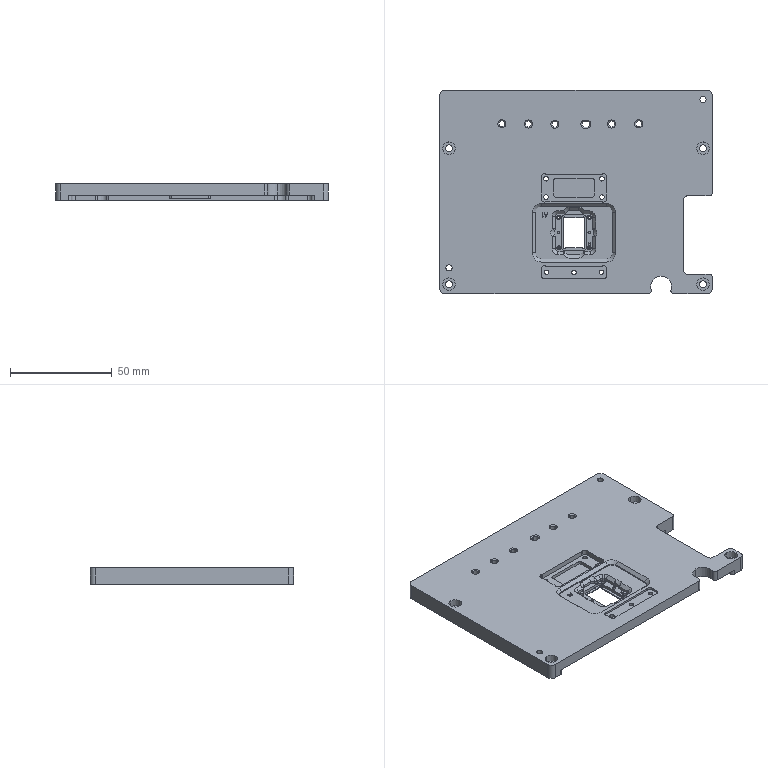NC program | NX | posted with a generic post | part box 134 x 100 x 8 mm
Lines 3064 to 4014 of 16793:
(ZLEVEL_PROFILE_COPY_COPY_COPY_1_COPY_COPY_1_COPY_COPY_COPY_1_COPY_COPY_COPY_1 )
N6066 T17 M6
N6068 G54
N6070 G17 G0 G90 X-14.25 Y-0.808 S9500 M3
N6072 G43 Z30. H17
N6074 Z-0.247
N6076 G94 G1 X-14.85 Y-1.155 F1000.
N6078 G3 X-15.05 Y-1.501 R0.4
N6080 G1 Y-2.49 F1100.
N6082 G2 X-15.074 Y-2.819 R2.3
N6084 X-14.802 Y-2.8 R2.
N6086 G1 X-13.751
N6088 G3 X-13.405 Y-2.6 R0.4
N6090 G1 X-13.058 Y-2.
N6092 G0 X-14.25 Y-0.808 Z-0.436
N6094 G1 X-14.85 Y-1.155 F1000.
N6096 G3 X-15.05 Y-1.501 R0.4
N6098 G1 Y-2.49 F1100.
N6100 G2 X-15.074 Y-2.819 R2.3
N6102 X-14.802 Y-2.8 R2.
N6104 G1 X-13.751
N6106 G3 X-13.405 Y-2.6 R0.4
N6108 G1 X-13.058 Y-2.
N6110 G0 X-14.25 Y-0.808 Z-0.624
N6112 G1 X-14.85 Y-1.155 F1000.
N6114 G3 X-15.05 Y-1.501 R0.4
N6116 G1 Y-2.49 F1100.
N6118 G2 X-15.074 Y-2.819 R2.3
N6120 X-14.802 Y-2.8 R2.
N6122 G1 X-13.751
N6124 G3 X-13.405 Y-2.6 R0.4
N6126 G1 X-13.058 Y-2.
N6128 G0 X-14.25 Y-0.808 Z-0.812
N6130 G1 X-14.85 Y-1.155 F1000.
N6132 G3 X-15.05 Y-1.501 R0.4
N6134 G1 Y-2.49 F1100.
N6136 G2 X-15.074 Y-2.819 R2.3
N6138 X-14.802 Y-2.8 R2.
N6140 G1 X-13.751
N6142 G3 X-13.405 Y-2.6 R0.4
N6144 G1 X-13.058 Y-2.
N6146 G0 X-14.25 Y-0.808 Z-1.
N6148 G1 X-14.85 Y-1.155 F1000.
N6150 G3 X-15.05 Y-1.501 R0.4
N6152 G1 Y-2.49 F1100.
N6154 G2 X-15.074 Y-2.819 R2.3
N6156 X-14.802 Y-2.8 R2.
N6158 G1 X-13.751
N6160 G3 X-13.405 Y-2.6 R0.4
N6162 G1 X-13.058 Y-2.
N6164 G0 X-14.25 Y-0.808 Z-1.247
N6166 G1 X-14.85 Y-1.155 F1000.
N6168 G3 X-15.05 Y-1.501 R0.4
N6170 G1 Y-2.49 F1100.
N6172 G2 X-15.074 Y-2.819 R2.3
N6174 X-14.802 Y-2.8 R2.
N6176 G1 X-13.751
N6178 G3 X-13.405 Y-2.6 R0.4
N6180 G1 X-13.058 Y-2.
N6182 G0 X-14.25 Y-0.808 Z-1.436
N6184 G1 X-14.85 Y-1.155 F1000.
N6186 G3 X-15.05 Y-1.501 R0.4
N6188 G1 Y-2.49 F1100.
N6190 G2 X-15.074 Y-2.819 R2.3
N6192 X-14.802 Y-2.8 R2.
N6194 G1 X-13.751
N6196 G3 X-13.405 Y-2.6 R0.4
N6198 G1 X-13.058 Y-2.
N6200 G0 X-14.25 Y-0.808 Z-1.76
N6202 G1 X-14.85 Y-1.155 F1000.
N6204 G3 X-15.05 Y-1.501 R0.4
N6206 G1 Y-2.49 F1100.
N6208 G2 X-15.074 Y-2.819 R2.3
N6210 X-14.802 Y-2.8 R2.
N6212 G1 X-13.751
N6214 G3 X-13.405 Y-2.6 R0.4
N6216 G1 X-13.058 Y-2.
N6218 G0 X-14.25 Y-0.808 Z-2.
N6220 G1 X-14.85 Y-1.155 F1000.
N6222 G3 X-15.05 Y-1.501 R0.4
N6224 G1 Y-2.49 F1100.
N6226 G2 X-15.074 Y-2.819 R2.3
N6228 X-14.802 Y-2.8 R2.
N6230 G1 X-13.751
N6232 G3 X-13.405 Y-2.6 R0.4
N6234 G1 X-13.058 Y-2.
N6236 G0 X-14.25 Y-0.808 Z-2.1
N6238 G1 X-14.85 Y-1.155 F1000.
N6240 G3 X-15.05 Y-1.501 R0.4
N6242 G1 Y-2.49 F1100.
N6244 G2 X-15.074 Y-2.819 R2.3
N6246 X-14.802 Y-2.8 R2.
N6248 G1 X-13.751
N6250 G3 X-13.405 Y-2.6 R0.4
N6252 G1 X-13.058 Y-2.
N6254 G0 X-14.25 Y-0.808 Z-2.267
N6256 G1 X-14.85 Y-1.155 F1000.
N6258 G3 X-15.05 Y-1.501 R0.4
N6260 G1 Y-2.49 F1100.
N6262 G2 X-15.074 Y-2.819 R2.3
N6264 X-14.802 Y-2.8 R2.
N6266 G1 X-13.751
N6268 G3 X-13.405 Y-2.6 R0.4
N6270 G1 X-13.058 Y-2.
N6272 G0 X-14.25 Y-0.808 Z-2.433
N6274 G1 X-14.85 Y-1.155 F1000.
N6276 G3 X-15.05 Y-1.501 R0.4
N6278 G1 Y-2.49 F1100.
N6280 G2 X-15.074 Y-2.819 R2.3
N6282 X-14.802 Y-2.8 R2.
N6284 G1 X-13.751
N6286 G3 X-13.405 Y-2.6 R0.4
N6288 G1 X-13.058 Y-2.
N6290 G0 X-14.25 Y-0.808 Z-2.6
N6292 G1 X-14.85 Y-1.155 F1000.
N6294 G3 X-15.05 Y-1.501 R0.4
N6296 G1 Y-2.49 F1100.
N6298 G2 X-15.074 Y-2.819 R2.3
N6300 X-14.802 Y-2.8 R2.
N6302 G1 X-13.751
N6304 G3 X-13.405 Y-2.6 R0.4
N6306 G1 X-13.058 Y-2.
N6308 G0 Z30.
N6310 X-8.2 Y1.492
N6312 Z-2.825
N6314 G1 X-8.8 Y1.145 F1000.
N6316 G3 X-9. Y0.799 R0.4
N6318 G1 Y-0.5 F1100.
N6320 X-7.701
N6322 G3 X-7.355 Y-0.3 R0.4
N6324 G1 X-7.008 Y0.3
N6326 G0 X-8.2 Y1.492 Z-3.05
N6328 G1 X-8.8 Y1.145 F1000.
N6330 G3 X-9. Y0.799 R0.4
N6332 G1 Y-0.5 F1100.
N6334 X-7.701
N6336 G3 X-7.355 Y-0.3 R0.4
N6338 G1 X-7.008 Y0.3
N6340 G0 X-8.2 Y1.492 Z-3.275
N6342 G1 X-8.8 Y1.145 F1000.
N6344 G3 X-9. Y0.799 R0.4
N6346 G1 Y-0.5 F1100.
N6348 X-7.701
N6350 G3 X-7.355 Y-0.3 R0.4
N6352 G1 X-7.008 Y0.3
N6354 G0 X-8.2 Y1.492 Z-3.5
N6356 G1 X-8.8 Y1.145 F1000.
N6358 G3 X-9. Y0.799 R0.4
N6360 G1 Y-0.5 F1100.
N6362 X-7.701
N6364 G3 X-7.355 Y-0.3 R0.4
N6366 G1 X-7.008 Y0.3
N6368 G0 X-8.2 Y1.492 Z-3.85
N6370 G1 X-8.8 Y1.145 F1000.
N6372 G3 X-9. Y0.799 R0.4
N6374 G1 Y-0.5 F1100.
N6376 X-7.701
N6378 G3 X-7.355 Y-0.3 R0.4
N6380 G1 X-7.008 Y0.3
N6382 G0 X-8.2 Y1.492 Z-4.05
N6384 G1 X-8.8 Y1.145 F1000.
N6386 G3 X-9. Y0.799 R0.4
N6388 G1 Y-0.5 F1100.
N6390 X-7.701
N6392 G3 X-7.355 Y-0.3 R0.4
N6394 G1 X-7.008 Y0.3
N6396 G0 X-8.2 Y1.492 Z-4.2
N6398 G1 X-8.8 Y1.145 F1000.
N6400 G3 X-9. Y0.799 R0.4
N6402 G1 Y-0.5 F1100.
N6404 X-7.701
N6406 G3 X-7.355 Y-0.3 R0.4
N6408 G1 X-7.008 Y0.3
N6410 G0 Z30.
N6412 X11.058 Y-2.
N6414 Z-0.247
N6416 G1 X11.404 Y-2.6 F1000.
N6418 G3 X11.751 Y-2.8 R0.4
N6420 G1 X12.74 F1100.
N6422 G2 X13.074 Y-2.824 R2.3
N6424 X13.05 Y-2.49 R2.3
N6426 G1 Y-1.501
N6428 G3 X12.85 Y-1.154 R0.4
N6430 G1 X12.25 Y-0.808
N6432 G0 X11.058 Y-2. Z-0.436
N6434 G1 X11.404 Y-2.6 F1000.
N6436 G3 X11.751 Y-2.8 R0.4
N6438 G1 X12.74 F1100.
N6440 G2 X13.074 Y-2.824 R2.3
N6442 X13.05 Y-2.49 R2.3
N6444 G1 Y-1.501
N6446 G3 X12.85 Y-1.154 R0.4
N6448 G1 X12.25 Y-0.808
N6450 G0 X11.057 Y-2. Z-0.624
N6452 G1 X11.404 Y-2.6 F1000.
N6454 G3 X11.75 Y-2.8 R0.4
N6456 G1 X12.74 F1100.
N6458 G2 X13.074 Y-2.824 R2.3
N6460 X13.05 Y-2.49 R2.3
N6462 G1 Y-1.5
N6464 G3 X12.85 Y-1.154 R0.4
N6466 G1 X12.25 Y-0.807
N6468 G0 X11.057 Y-2. Z-0.812
N6470 G1 X11.404 Y-2.6 F1000.
N6472 G3 X11.75 Y-2.8 R0.4
N6474 G1 X12.74 F1100.
N6476 G2 X13.074 Y-2.824 R2.3
N6478 X13.05 Y-2.49 R2.3
N6480 G1 Y-1.5
N6482 G3 X12.85 Y-1.154 R0.4
N6484 G1 X12.25 Y-0.807
N6486 G0 X11.057 Y-2. Z-1.
N6488 G1 X11.404 Y-2.6 F1000.
N6490 G3 X11.75 Y-2.8 R0.4
N6492 G1 X12.74 F1100.
N6494 G2 X13.074 Y-2.824 R2.3
N6496 X13.05 Y-2.49 R2.3
N6498 G1 Y-1.5
N6500 G3 X12.85 Y-1.154 R0.4
N6502 G1 X12.25 Y-0.807
N6504 G0 X11.057 Y-2. Z-1.247
N6506 G1 X11.403 Y-2.6 F1000.
N6508 G3 X11.75 Y-2.8 R0.4
N6510 G1 X12.74 F1100.
N6512 G2 X13.074 Y-2.824 R2.3
N6514 X13.05 Y-2.49 R2.3
N6516 G1 Y-1.5
N6518 G3 X12.85 Y-1.153 R0.4
N6520 G1 X12.25 Y-0.807
N6522 G0 X11.057 Y-2. Z-1.436
N6524 G1 X11.403 Y-2.6 F1000.
N6526 G3 X11.749 Y-2.8 R0.4
N6528 G1 X12.74 F1100.
N6530 G2 X13.074 Y-2.824 R2.3
N6532 X13.05 Y-2.49 R2.3
N6534 G1 Y-1.499
N6536 G3 X12.85 Y-1.153 R0.4
N6538 G1 X12.25 Y-0.807
N6540 G0 X11.056 Y-2. Z-1.76
N6542 G1 X11.403 Y-2.6 F1000.
N6544 G3 X11.749 Y-2.8 R0.4
N6546 G1 X12.74 F1100.
N6548 G2 X13.074 Y-2.824 R2.3
N6550 X13.05 Y-2.49 R2.3
N6552 G1 Y-1.499
N6554 G3 X12.85 Y-1.153 R0.4
N6556 G1 X12.25 Y-0.806
N6558 G0 X11.056 Y-2. Z-2.
N6560 G1 X11.402 Y-2.6 F1000.
N6562 G3 X11.749 Y-2.8 R0.4
N6564 G1 X12.74 F1100.
N6566 G2 X13.074 Y-2.824 R2.3
N6568 X13.05 Y-2.49 R2.3
N6570 G1 Y-1.499
N6572 G3 X12.85 Y-1.152 R0.4
N6574 G1 X12.25 Y-0.806
N6576 G0 X11.056 Y-2. Z-2.1
N6578 G1 X11.402 Y-2.6 F1000.
N6580 G3 X11.749 Y-2.8 R0.4
N6582 G1 X12.74 F1100.
N6584 G2 X13.074 Y-2.824 R2.3
N6586 X13.05 Y-2.49 R2.3
N6588 G1 Y-1.499
N6590 G3 X12.85 Y-1.152 R0.4
N6592 G1 X12.25 Y-0.806
N6594 G0 X11.056 Y-2. Z-2.267
N6596 G1 X11.402 Y-2.6 F1000.
N6598 G3 X11.749 Y-2.8 R0.4
N6600 G1 X12.74 F1100.
N6602 G2 X13.074 Y-2.824 R2.3
N6604 X13.05 Y-2.49 R2.3
N6606 G1 Y-1.499
N6608 G3 X12.85 Y-1.152 R0.4
N6610 G1 X12.25 Y-0.806
N6612 G0 X11.056 Y-2. Z-2.433
N6614 G1 X11.402 Y-2.6 F1000.
N6616 G3 X11.748 Y-2.8 R0.4
N6618 G1 X12.74 F1100.
N6620 G2 X13.074 Y-2.824 R2.3
N6622 X13.05 Y-2.49 R2.3
N6624 G1 Y-1.498
N6626 G3 X12.85 Y-1.152 R0.4
N6628 G1 X12.25 Y-0.806
N6630 G0 X11.055 Y-2. Z-2.6
N6632 G1 X11.402 Y-2.6 F1000.
N6634 G3 X11.748 Y-2.8 R0.4
N6636 G1 X12.74 F1100.
N6638 G2 X13.074 Y-2.824 R2.3
N6640 X13.05 Y-2.49 R2.3
N6642 G1 Y-1.498
N6644 G3 X12.85 Y-1.152 R0.4
N6646 G1 X12.25 Y-0.805
N6648 G0 Z30.
N6650 X5.008 Y0.3
N6652 Z-2.825
N6654 G1 X5.355 Y-0.3 F1000.
N6656 G3 X5.701 Y-0.5 R0.4
N6658 G1 X7. F1100.
N6660 Y0.799
N6662 G3 X6.8 Y1.145 R0.4
N6664 G1 X6.2 Y1.492
N6666 G0 X5.008 Y0.3 Z-3.05
N6668 G1 X5.355 Y-0.3 F1000.
N6670 G3 X5.701 Y-0.5 R0.4
N6672 G1 X7. F1100.
N6674 Y0.799
N6676 G3 X6.8 Y1.145 R0.4
N6678 G1 X6.2 Y1.492
N6680 G0 X5.008 Y0.3 Z-3.275
N6682 G1 X5.355 Y-0.3 F1000.
N6684 G3 X5.701 Y-0.5 R0.4
N6686 G1 X7. F1100.
N6688 Y0.799
N6690 G3 X6.8 Y1.145 R0.4
N6692 G1 X6.2 Y1.492
N6694 G0 X5.008 Y0.3 Z-3.5
N6696 G1 X5.355 Y-0.3 F1000.
N6698 G3 X5.701 Y-0.5 R0.4
N6700 G1 X7. F1100.
N6702 Y0.799
N6704 G3 X6.8 Y1.145 R0.4
N6706 G1 X6.2 Y1.492
N6708 G0 X5.008 Y0.3 Z-3.85
N6710 G1 X5.355 Y-0.3 F1000.
N6712 G3 X5.701 Y-0.5 R0.4
N6714 G1 X7. F1100.
N6716 Y0.799
N6718 G3 X6.8 Y1.145 R0.4
N6720 G1 X6.2 Y1.492
N6722 G0 X5.008 Y0.3 Z-4.05
N6724 G1 X5.355 Y-0.3 F1000.
N6726 G3 X5.701 Y-0.5 R0.4
N6728 G1 X7. F1100.
N6730 Y0.799
N6732 G3 X6.8 Y1.145 R0.4
N6734 G1 X6.2 Y1.492
N6736 G0 X5.008 Y0.3 Z-4.2
N6738 G1 X5.355 Y-0.3 F1000.
N6740 G3 X5.701 Y-0.5 R0.4
N6742 G1 X7. F1100.
N6744 Y0.799
N6746 G3 X6.8 Y1.145 R0.4
N6748 G1 X6.2 Y1.492
N6750 G0 Z30.
N6752 X12.25 Y4.808
N6754 Z-0.247
N6756 G1 X12.85 Y5.155 F1000.
N6758 G3 X13.05 Y5.501 R0.4
N6760 G1 Y6.49 F1100.
N6762 G2 X13.074 Y6.824 R2.3
N6764 X12.74 Y6.8 R2.3
N6766 G1 X11.751
N6768 G3 X11.405 Y6.6 R0.4
N6770 G1 X11.058 Y6.
N6772 G0 X12.25 Y4.808 Z-0.436
N6774 G1 X12.85 Y5.155 F1000.
N6776 G3 X13.05 Y5.501 R0.4
N6778 G1 Y6.49 F1100.
N6780 G2 X13.074 Y6.824 R2.3
N6782 X12.74 Y6.8 R2.3
N6784 G1 X11.751
N6786 G3 X11.405 Y6.6 R0.4
N6788 G1 X11.058 Y6.
N6790 G0 X12.25 Y4.808 Z-0.624
N6792 G1 X12.85 Y5.155 F1000.
N6794 G3 X13.05 Y5.501 R0.4
N6796 G1 Y6.49 F1100.
N6798 G2 X13.074 Y6.824 R2.3
N6800 X12.74 Y6.8 R2.3
N6802 G1 X11.751
N6804 G3 X11.405 Y6.6 R0.4
N6806 G1 X11.058 Y6.
N6808 G0 X12.25 Y4.808 Z-0.812
N6810 G1 X12.85 Y5.155 F1000.
N6812 G3 X13.05 Y5.501 R0.4
N6814 G1 Y6.49 F1100.
N6816 G2 X13.074 Y6.824 R2.3
N6818 X12.74 Y6.8 R2.3
N6820 G1 X11.751
N6822 G3 X11.405 Y6.6 R0.4
N6824 G1 X11.058 Y6.
N6826 G0 X12.25 Y4.808 Z-1.
N6828 G1 X12.85 Y5.155 F1000.
N6830 G3 X13.05 Y5.501 R0.4
N6832 G1 Y6.49 F1100.
N6834 G2 X13.074 Y6.824 R2.3
N6836 X12.74 Y6.8 R2.3
N6838 G1 X11.751
N6840 G3 X11.405 Y6.6 R0.4
N6842 G1 X11.058 Y6.
N6844 G0 X12.25 Y4.808 Z-1.247
N6846 G1 X12.85 Y5.155 F1000.
N6848 G3 X13.05 Y5.501 R0.4
N6850 G1 Y6.49 F1100.
N6852 G2 X13.074 Y6.824 R2.3
N6854 X12.74 Y6.8 R2.3
N6856 G1 X11.751
N6858 G3 X11.405 Y6.6 R0.4
N6860 G1 X11.058 Y6.
N6862 G0 X12.25 Y4.808 Z-1.436
N6864 G1 X12.85 Y5.155 F1000.
N6866 G3 X13.05 Y5.501 R0.4
N6868 G1 Y6.49 F1100.
N6870 G2 X13.074 Y6.824 R2.3
N6872 X12.74 Y6.8 R2.3
N6874 G1 X11.751
N6876 G3 X11.405 Y6.6 R0.4
N6878 G1 X11.058 Y6.
N6880 G0 X12.25 Y4.808 Z-1.76
N6882 G1 X12.85 Y5.155 F1000.
N6884 G3 X13.05 Y5.501 R0.4
N6886 G1 Y6.49 F1100.
N6888 G2 X13.074 Y6.824 R2.3
N6890 X12.74 Y6.8 R2.3
N6892 G1 X11.751
N6894 G3 X11.405 Y6.6 R0.4
N6896 G1 X11.058 Y6.
N6898 G0 X12.25 Y4.808 Z-2.
N6900 G1 X12.85 Y5.155 F1000.
N6902 G3 X13.05 Y5.501 R0.4
N6904 G1 Y6.49 F1100.
N6906 G2 X13.074 Y6.824 R2.3
N6908 X12.74 Y6.8 R2.3
N6910 G1 X11.751
N6912 G3 X11.405 Y6.6 R0.4
N6914 G1 X11.058 Y6.
N6916 G0 X12.25 Y4.808 Z-2.1
N6918 G1 X12.85 Y5.155 F1000.
N6920 G3 X13.05 Y5.501 R0.4
N6922 G1 Y6.49 F1100.
N6924 G2 X13.074 Y6.824 R2.3
N6926 X12.74 Y6.8 R2.3
N6928 G1 X11.751
N6930 G3 X11.405 Y6.6 R0.4
N6932 G1 X11.058 Y6.
N6934 G0 X12.25 Y4.808 Z-2.267
N6936 G1 X12.85 Y5.155 F1000.
N6938 G3 X13.05 Y5.501 R0.4
N6940 G1 Y6.49 F1100.
N6942 G2 X13.074 Y6.824 R2.3
N6944 X12.74 Y6.8 R2.3
N6946 G1 X11.751
N6948 G3 X11.405 Y6.6 R0.4
N6950 G1 X11.058 Y6.
N6952 G0 X12.25 Y4.808 Z-2.433
N6954 G1 X12.85 Y5.155 F1000.
N6956 G3 X13.05 Y5.501 R0.4
N6958 G1 Y6.49 F1100.
N6960 G2 X13.074 Y6.824 R2.3
N6962 X12.74 Y6.8 R2.3
N6964 G1 X11.751
N6966 G3 X11.405 Y6.6 R0.4
N6968 G1 X11.058 Y6.
N6970 G0 X12.25 Y4.808 Z-2.6
N6972 G1 X12.85 Y5.155 F1000.
N6974 G3 X13.05 Y5.501 R0.4
N6976 G1 Y6.49 F1100.
N6978 G2 X13.074 Y6.824 R2.3
N6980 X12.74 Y6.8 R2.3
N6982 G1 X11.751
N6984 G3 X11.405 Y6.6 R0.4
N6986 G1 X11.058 Y6.
N6988 G0 Z30.
N6990 X6.2 Y2.508
N6992 Z-2.825
N6994 G1 X6.8 Y2.855 F1000.
N6996 G3 X7. Y3.201 R0.4
N6998 G1 Y4.5 F1100.
N7000 X5.701
N7002 G3 X5.355 Y4.3 R0.4
N7004 G1 X5.008 Y3.7
N7006 G0 X6.2 Y2.508 Z-3.05
N7008 G1 X6.8 Y2.855 F1000.
N7010 G3 X7. Y3.201 R0.4
N7012 G1 Y4.5 F1100.
N7014 X5.701
N7016 G3 X5.355 Y4.3 R0.4
N7018 G1 X5.008 Y3.7
N7020 G0 X6.2 Y2.508 Z-3.275
N7022 G1 X6.8 Y2.855 F1000.
N7024 G3 X7. Y3.201 R0.4
N7026 G1 Y4.5 F1100.
N7028 X5.701
N7030 G3 X5.355 Y4.3 R0.4
N7032 G1 X5.008 Y3.7
N7034 G0 X6.2 Y2.508 Z-3.5
N7036 G1 X6.8 Y2.855 F1000.
N7038 G3 X7. Y3.201 R0.4
N7040 G1 Y4.5 F1100.
N7042 X5.701
N7044 G3 X5.355 Y4.3 R0.4
N7046 G1 X5.008 Y3.7
N7048 G0 X6.2 Y2.508 Z-3.85
N7050 G1 X6.8 Y2.855 F1000.
N7052 G3 X7. Y3.201 R0.4
N7054 G1 Y4.5 F1100.
N7056 X5.701
N7058 G3 X5.355 Y4.3 R0.4
N7060 G1 X5.008 Y3.7
N7062 G0 X6.2 Y2.508 Z-4.05
N7064 G1 X6.8 Y2.855 F1000.
N7066 G3 X7. Y3.201 R0.4
N7068 G1 Y4.5 F1100.
N7070 X5.701
N7072 G3 X5.355 Y4.3 R0.4
N7074 G1 X5.008 Y3.7
N7076 G0 X6.2 Y2.508 Z-4.2
N7078 G1 X6.8 Y2.855 F1000.
N7080 G3 X7. Y3.201 R0.4
N7082 G1 Y4.5 F1100.
N7084 X5.701
N7086 G3 X5.355 Y4.3 R0.4
N7088 G1 X5.008 Y3.7
N7090 G0 Z30.
N7092 X-13.058 Y6.
N7094 Z-0.247
N7096 G1 X-13.405 Y6.6 F1000.
N7098 G3 X-13.751 Y6.8 R0.4
N7100 G1 X-14.74 F1100.
N7102 G2 X-15.074 Y6.824 R2.3
N7104 X-15.05 Y6.49 R2.3
N7106 G1 Y5.501
N7108 G3 X-14.85 Y5.155 R0.4
N7110 G1 X-14.25 Y4.808
N7112 G0 X-13.058 Y6. Z-0.436
N7114 G1 X-13.405 Y6.6 F1000.
N7116 G3 X-13.751 Y6.8 R0.4
N7118 G1 X-14.74 F1100.
N7120 G2 X-15.074 Y6.824 R2.3
N7122 X-15.05 Y6.49 R2.3
N7124 G1 Y5.501
N7126 G3 X-14.85 Y5.155 R0.4
N7128 G1 X-14.25 Y4.808
N7130 G0 X-13.058 Y6. Z-0.624
N7132 G1 X-13.405 Y6.6 F1000.
N7134 G3 X-13.751 Y6.8 R0.4
N7136 G1 X-14.74 F1100.
N7138 G2 X-15.074 Y6.824 R2.3
N7140 X-15.05 Y6.49 R2.3
N7142 G1 Y5.501
N7144 G3 X-14.85 Y5.155 R0.4
N7146 G1 X-14.25 Y4.808
N7148 G0 X-13.058 Y6. Z-0.812
N7150 G1 X-13.405 Y6.6 F1000.
N7152 G3 X-13.751 Y6.8 R0.4
N7154 G1 X-14.74 F1100.
N7156 G2 X-15.074 Y6.824 R2.3
N7158 X-15.05 Y6.49 R2.3
N7160 G1 Y5.501
N7162 G3 X-14.85 Y5.155 R0.4
N7164 G1 X-14.25 Y4.808
N7166 G0 X-13.058 Y6. Z-1.
N7168 G1 X-13.405 Y6.6 F1000.
N7170 G3 X-13.751 Y6.8 R0.4
N7172 G1 X-14.74 F1100.
N7174 G2 X-15.074 Y6.824 R2.3
N7176 X-15.05 Y6.49 R2.3
N7178 G1 Y5.501
N7180 G3 X-14.85 Y5.155 R0.4
N7182 G1 X-14.25 Y4.808
N7184 G0 X-13.058 Y6. Z-1.247
N7186 G1 X-13.405 Y6.6 F1000.
N7188 G3 X-13.751 Y6.8 R0.4
N7190 G1 X-14.74 F1100.
N7192 G2 X-15.074 Y6.824 R2.3
N7194 X-15.05 Y6.49 R2.3
N7196 G1 Y5.501
N7198 G3 X-14.85 Y5.155 R0.4
N7200 G1 X-14.25 Y4.808
N7202 G0 X-13.058 Y6. Z-1.436
N7204 G1 X-13.405 Y6.6 F1000.
N7206 G3 X-13.751 Y6.8 R0.4
N7208 G1 X-14.74 F1100.
N7210 G2 X-15.074 Y6.824 R2.3
N7212 X-15.05 Y6.49 R2.3
N7214 G1 Y5.501
N7216 G3 X-14.85 Y5.155 R0.4
N7218 G1 X-14.25 Y4.808
N7220 G0 X-13.058 Y6. Z-1.76
N7222 G1 X-13.405 Y6.6 F1000.
N7224 G3 X-13.751 Y6.8 R0.4
N7226 G1 X-14.74 F1100.
N7228 G2 X-15.074 Y6.824 R2.3
N7230 X-15.05 Y6.49 R2.3
N7232 G1 Y5.501
N7234 G3 X-14.85 Y5.155 R0.4
N7236 G1 X-14.25 Y4.808
N7238 G0 X-13.058 Y6. Z-2.
N7240 G1 X-13.405 Y6.6 F1000.
N7242 G3 X-13.751 Y6.8 R0.4
N7244 G1 X-14.74 F1100.
N7246 G2 X-15.074 Y6.824 R2.3
N7248 X-15.05 Y6.49 R2.3
N7250 G1 Y5.501
N7252 G3 X-14.85 Y5.155 R0.4
N7254 G1 X-14.25 Y4.808
N7256 G0 X-13.058 Y6. Z-2.1
N7258 G1 X-13.405 Y6.6 F1000.
N7260 G3 X-13.751 Y6.8 R0.4
N7262 G1 X-14.74 F1100.
N7264 G2 X-15.074 Y6.824 R2.3
N7266 X-15.05 Y6.49 R2.3
N7268 G1 Y5.501
N7270 G3 X-14.85 Y5.155 R0.4
N7272 G1 X-14.25 Y4.808
N7274 G0 X-13.058 Y6. Z-2.267
N7276 G1 X-13.405 Y6.6 F1000.
N7278 G3 X-13.751 Y6.8 R0.4
N7280 G1 X-14.74 F1100.
N7282 G2 X-15.074 Y6.824 R2.3
N7284 X-15.05 Y6.49 R2.3
N7286 G1 Y5.501
N7288 G3 X-14.85 Y5.155 R0.4
N7290 G1 X-14.25 Y4.808
N7292 G0 X-13.058 Y6. Z-2.433
N7294 G1 X-13.405 Y6.6 F1000.
N7296 G3 X-13.751 Y6.8 R0.4
N7298 G1 X-14.74 F1100.
N7300 G2 X-15.074 Y6.824 R2.3
N7302 X-15.05 Y6.49 R2.3
N7304 G1 Y5.501
N7306 G3 X-14.85 Y5.155 R0.4
N7308 G1 X-14.25 Y4.808
N7310 G0 X-13.058 Y6. Z-2.6
N7312 G1 X-13.405 Y6.6 F1000.
N7314 G3 X-13.751 Y6.8 R0.4
N7316 G1 X-14.74 F1100.
N7318 G2 X-15.074 Y6.824 R2.3
N7320 X-15.05 Y6.49 R2.3
N7322 G1 Y5.501
N7324 G3 X-14.85 Y5.155 R0.4
N7326 G1 X-14.25 Y4.808
N7328 G0 Z30.
N7330 X-7.008 Y3.7
N7332 Z-2.825
N7334 G1 X-7.355 Y4.3 F1000.
N7336 G3 X-7.701 Y4.5 R0.4
N7338 G1 X-9. F1100.
N7340 Y3.201
N7342 G3 X-8.8 Y2.855 R0.4
N7344 G1 X-8.2 Y2.508
N7346 G0 X-7.008 Y3.7 Z-3.05
N7348 G1 X-7.355 Y4.3 F1000.
N7350 G3 X-7.701 Y4.5 R0.4
N7352 G1 X-9. F1100.
N7354 Y3.201
N7356 G3 X-8.8 Y2.855 R0.4
N7358 G1 X-8.2 Y2.508
N7360 G0 X-7.008 Y3.7 Z-3.275
N7362 G1 X-7.355 Y4.3 F1000.
N7364 G3 X-7.701 Y4.5 R0.4
N7366 G1 X-9. F1100.
N7368 Y3.201
N7370 G3 X-8.8 Y2.855 R0.4
N7372 G1 X-8.2 Y2.508
N7374 G0 X-7.008 Y3.7 Z-3.5
N7376 G1 X-7.355 Y4.3 F1000.
N7378 G3 X-7.701 Y4.5 R0.4
N7380 G1 X-9. F1100.
N7382 Y3.201
N7384 G3 X-8.8 Y2.855 R0.4
N7386 G1 X-8.2 Y2.508
N7388 G0 X-7.008 Y3.7 Z-3.85
N7390 G1 X-7.355 Y4.3 F1000.
N7392 G3 X-7.701 Y4.5 R0.4
N7394 G1 X-9. F1100.
N7396 Y3.201
N7398 G3 X-8.8 Y2.855 R0.4
N7400 G1 X-8.2 Y2.508
N7402 G0 X-7.008 Y3.7 Z-4.05
N7404 G1 X-7.355 Y4.3 F1000.
N7406 G3 X-7.701 Y4.5 R0.4
N7408 G1 X-9. F1100.
N7410 Y3.201
N7412 G3 X-8.8 Y2.855 R0.4
N7414 G1 X-8.2 Y2.508
N7416 G0 X-7.008 Y3.7 Z-4.2
N7418 G1 X-7.355 Y4.3 F1000.
N7420 G3 X-7.701 Y4.5 R0.4
N7422 G1 X-9. F1100.
N7424 Y3.201
N7426 G3 X-8.8 Y2.855 R0.4
N7428 G1 X-8.2 Y2.508
N7430 G0 Z30.
N7432 X-13.058 Y-39.25
N7434 Z-0.247
N7436 G1 X-13.405 Y-38.65 F1000.
N7438 G3 X-13.751 Y-38.45 R0.4
N7440 G1 X-14.74 F1100.
N7442 G2 X-15.074 Y-38.426 R2.3
N7444 X-15.05 Y-38.76 R2.3
N7446 G1 Y-40.24
N7448 X-15.057 Y-40.413
N7450 X-15.076 Y-40.575
N7452 G2 X-14.74 Y-40.55 R2.3
N7454 G1 X-13.751
N7456 G3 X-13.405 Y-40.35 R0.4
N7458 G1 X-13.058 Y-39.75
N7460 G0 Y-39.25 Z-0.436
N7462 G1 X-13.405 Y-38.65 F1000.
N7464 G3 X-13.751 Y-38.45 R0.4
N7466 G1 X-14.74 F1100.
N7468 G2 X-15.074 Y-38.426 R2.3
N7470 X-15.05 Y-38.76 R2.3
N7472 G1 Y-40.24
N7474 X-15.057 Y-40.414
N7476 X-15.075 Y-40.575
N7478 G2 X-14.74 Y-40.55 R2.3
N7480 G1 X-13.751
N7482 G3 X-13.405 Y-40.35 R0.4
N7484 G1 X-13.058 Y-39.75
N7486 G0 Y-39.25 Z-0.624
N7488 G1 X-13.405 Y-38.65 F1000.
N7490 G3 X-13.751 Y-38.45 R0.4
N7492 G1 X-14.74 F1100.
N7494 G2 X-15.074 Y-38.426 R2.3
N7496 X-15.05 Y-38.76 R2.3
N7498 G1 Y-40.24
N7500 X-15.057 Y-40.414
N7502 X-15.075 Y-40.574
N7504 G2 X-14.74 Y-40.55 R2.3
N7506 G1 X-13.751
N7508 G3 X-13.405 Y-40.35 R0.4
N7510 G1 X-13.058 Y-39.75
N7512 G0 Y-39.25 Z-0.812
N7514 G1 X-13.405 Y-38.65 F1000.
N7516 G3 X-13.751 Y-38.45 R0.4
N7518 G1 X-14.74 F1100.
N7520 G2 X-15.074 Y-38.426 R2.3
N7522 X-15.05 Y-38.76 R2.3
N7524 G1 Y-40.24
N7526 Y-40.286
N7528 X-15.074 Y-40.574
N7530 G2 X-14.74 Y-40.55 R2.3
N7532 G1 X-13.751
N7534 G3 X-13.405 Y-40.35 R0.4
N7536 G1 X-13.058 Y-39.75
N7538 G0 Y-39.25 Z-1.
N7540 G1 X-13.405 Y-38.65 F1000.
N7542 G3 X-13.751 Y-38.45 R0.4
N7544 G1 X-14.74 F1100.
N7546 G2 X-15.074 Y-38.426 R2.3
N7548 X-15.05 Y-38.76 R2.3
N7550 G1 Y-40.24
N7552 Y-40.286
N7554 X-15.074 Y-40.574
N7556 G2 X-14.74 Y-40.55 R2.3
N7558 G1 X-13.751
N7560 G3 X-13.405 Y-40.35 R0.4
N7562 G1 X-13.058 Y-39.75
N7564 G0 Z30.
N7566 X11.058
N7568 Z-0.247
N7570 G1 X11.405 Y-40.35 F1000.
N7572 G3 X11.751 Y-40.55 R0.4
N7574 G1 X12.74 F1100.
N7576 G2 X13.076 Y-40.575 R2.3
N7578 G1 X13.071 Y-40.548
N7580 G2 X13.05 Y-40.24 R2.3
N7582 G1 Y-38.76
N7584 G2 X13.074 Y-38.425 R2.3
N7586 G1 X13.041 Y-38.43
N7588 G2 X12.74 Y-38.45 R2.3
N7590 G1 X11.751
N7592 G3 X11.405 Y-38.65 R0.4
N7594 G1 X11.058 Y-39.25
N7596 G0 Y-39.75 Z-0.436
N7598 G1 X11.405 Y-40.35 F1000.
N7600 G3 X11.751 Y-40.55 R0.4
N7602 G1 X12.74 F1100.
N7604 G2 X13.075 Y-40.575 R2.3
N7606 G1 X13.071 Y-40.548
N7608 X13.057 Y-40.419
N7610 X13.053 Y-40.357
N7612 X13.05 Y-40.24
N7614 Y-38.76
N7616 G2 X13.074 Y-38.426 R2.3
N7618 G1 X13.041 Y-38.43
N7620 G2 X12.74 Y-38.45 R2.3
N7622 G1 X11.751
N7624 G3 X11.405 Y-38.65 R0.4
N7626 G1 X11.058 Y-39.25
N7628 G0 Y-39.75 Z-0.624
N7630 G1 X11.405 Y-40.35 F1000.
N7632 G3 X11.751 Y-40.55 R0.4
N7634 G1 X12.74 F1100.
N7636 G2 X13.075 Y-40.574 R2.3
N7638 G1 X13.071 Y-40.548
N7640 X13.057 Y-40.419
N7642 X13.053 Y-40.357
N7644 X13.05 Y-40.24
N7646 Y-38.76
N7648 G2 X13.074 Y-38.426 R2.3
N7650 G1 X13.041 Y-38.43
N7652 G2 X12.74 Y-38.45 R2.3
N7654 G1 X11.751
N7656 G3 X11.405 Y-38.65 R0.4
N7658 G1 X11.058 Y-39.25
N7660 G0 Y-39.75 Z-0.812
N7662 G1 X11.405 Y-40.35 F1000.
N7664 G3 X11.751 Y-40.55 R0.4
N7666 G1 X12.74 F1100.
N7668 G2 X13.074 Y-40.574 R2.3
N7670 G1 X13.068 Y-40.527
N7672 X13.057 Y-40.419
N7674 X13.053 Y-40.357
N7676 X13.05 Y-40.24
N7678 Y-38.76
N7680 G2 X13.074 Y-38.426 R2.3
N7682 G1 X13.072
N7684 G2 X12.74 Y-38.45 R2.3
N7686 G1 X11.751
N7688 G3 X11.405 Y-38.65 R0.4
N7690 G1 X11.058 Y-39.25
N7692 G0 Y-39.75 Z-1.
N7694 G1 X11.405 Y-40.35 F1000.
N7696 G3 X11.751 Y-40.55 R0.4
N7698 G1 X12.74 F1100.
N7700 G2 X13.074 Y-40.574 R2.3
N7702 G1 X13.068 Y-40.527
N7704 X13.057 Y-40.42
N7706 X13.053 Y-40.357
N7708 X13.05 Y-40.24
N7710 Y-38.76
N7712 G2 X13.074 Y-38.427 R2.3
N7714 G1 X13.072 Y-38.426
N7716 G2 X12.74 Y-38.45 R2.3
N7718 G1 X11.751
N7720 G3 X11.405 Y-38.65 R0.4
N7722 G1 X11.058 Y-39.25
N7724 G0 Z30.
N7726 X57.074 Y-4.731
N7728 Z-0.247
N7730 G1 X56.728 Y-4.131 F1000.
N7732 G3 X56.381 Y-3.931 R0.4
N7734 G1 X55.082 F1100.
N7736 Y-5.23
N7738 G3 X55.282 Y-5.577 R0.4
N7740 G1 X55.882 Y-5.923
N7742 G0 X57.074 Y-4.731 Z-0.436
N7744 G1 X56.728 Y-4.131 F1000.
N7746 G3 X56.381 Y-3.931 R0.4
N7748 G1 X55.082 F1100.
N7750 Y-5.23
N7752 G3 X55.282 Y-5.577 R0.4
N7754 G1 X55.882 Y-5.923
N7756 G0 X57.074 Y-4.731 Z-0.624
N7758 G1 X56.728 Y-4.131 F1000.
N7760 G3 X56.381 Y-3.931 R0.4
N7762 G1 X55.082 F1100.
N7764 Y-5.23
N7766 G3 X55.282 Y-5.577 R0.4
N7768 G1 X55.882 Y-5.923
N7770 G0 X57.074 Y-4.731 Z-0.812
N7772 G1 X56.728 Y-4.131 F1000.
N7774 G3 X56.381 Y-3.931 R0.4
N7776 G1 X55.082 F1100.
N7778 Y-5.23
N7780 G3 X55.282 Y-5.577 R0.4
N7782 G1 X55.882 Y-5.923
N7784 G0 X57.074 Y-4.731 Z-1.
N7786 G1 X56.728 Y-4.131 F1000.
N7788 G3 X56.381 Y-3.931 R0.4
N7790 G1 X55.082 F1100.
N7792 Y-5.23
N7794 G3 X55.282 Y-5.577 R0.4
N7796 G1 X55.882 Y-5.923
N7798 G0 X57.074 Y-4.731 Z-1.247
N7800 G1 X56.728 Y-4.131 F1000.
N7802 G3 X56.381 Y-3.931 R0.4
N7804 G1 X55.082 F1100.
N7806 Y-5.23
N7808 G3 X55.282 Y-5.577 R0.4
N7810 G1 X55.882 Y-5.923
N7812 G0 X57.074 Y-4.731 Z-1.436
N7814 G1 X56.728 Y-4.131 F1000.
N7816 G3 X56.381 Y-3.931 R0.4
N7818 G1 X55.082 F1100.
N7820 Y-5.23
N7822 G3 X55.282 Y-5.577 R0.4
N7824 G1 X55.882 Y-5.923
N7826 G0 X57.074 Y-4.731 Z-1.76
N7828 G1 X56.728 Y-4.131 F1000.
N7830 G3 X56.381 Y-3.931 R0.4
N7832 G1 X55.082 F1100.
N7834 Y-5.23
N7836 G3 X55.282 Y-5.577 R0.4
N7838 G1 X55.882 Y-5.923
N7840 G0 X57.074 Y-4.731 Z-2.
N7842 G1 X56.728 Y-4.131 F1000.
N7844 G3 X56.381 Y-3.931 R0.4
N7846 G1 X55.082 F1100.
N7848 Y-5.23
N7850 G3 X55.282 Y-5.577 R0.4
N7852 G1 X55.882 Y-5.923
N7854 G0 X57.074 Y-4.731 Z-2.1
N7856 G1 X56.728 Y-4.131 F1000.
N7858 G3 X56.381 Y-3.931 R0.4
N7860 G1 X55.082 F1100.
N7862 Y-5.23
N7864 G3 X55.282 Y-5.577 R0.4
N7866 G1 X55.882 Y-5.923
N7868 G0 X57.074 Y-4.731 Z-2.267
N7870 G1 X56.728 Y-4.131 F1000.
N7872 G3 X56.381 Y-3.931 R0.4
N7874 G1 X55.082 F1100.
N7876 Y-5.23
N7878 G3 X55.282 Y-5.577 R0.4
N7880 G1 X55.882 Y-5.923
N7882 G0 X57.074 Y-4.731 Z-2.433
N7884 G1 X56.728 Y-4.131 F1000.
N7886 G3 X56.381 Y-3.931 R0.4
N7888 G1 X55.082 F1100.
N7890 Y-5.23
N7892 G3 X55.282 Y-5.577 R0.4
N7894 G1 X55.882 Y-5.923
N7896 G0 X57.074 Y-4.731 Z-2.6
N7898 G1 X56.728 Y-4.131 F1000.
N7900 G3 X56.381 Y-3.931 R0.4
N7902 G1 X55.082 F1100.
N7904 Y-5.23
N7906 G3 X55.282 Y-5.577 R0.4
N7908 G1 X55.882 Y-5.923
N7910 G0 X57.074 Y-4.731 Z-2.825
N7912 G1 X56.728 Y-4.131 F1000.
N7914 G3 X56.381 Y-3.931 R0.4
N7916 G1 X55.082 F1100.
N7918 Y-5.23
N7920 G3 X55.282 Y-5.577 R0.4
N7922 G1 X55.882 Y-5.923
N7924 G0 X57.074 Y-4.731 Z-3.05
N7926 G1 X56.728 Y-4.131 F1000.
N7928 G3 X56.381 Y-3.931 R0.4
N7930 G1 X55.082 F1100.
N7932 Y-5.23
N7934 G3 X55.282 Y-5.577 R0.4
N7936 G1 X55.882 Y-5.923
N7938 G0 X57.074 Y-4.731 Z-3.275
N7940 G1 X56.728 Y-4.131 F1000.
N7942 G3 X56.381 Y-3.931 R0.4
N7944 G1 X55.082 F1100.
N7946 Y-5.23
N7948 G3 X55.282 Y-5.577 R0.4
N7950 G1 X55.882 Y-5.923
N7952 G0 X57.074 Y-4.731 Z-3.5
N7954 G1 X56.728 Y-4.131 F1000.
N7956 G3 X56.381 Y-3.931 R0.4
N7958 G1 X55.082 F1100.
N7960 Y-5.23